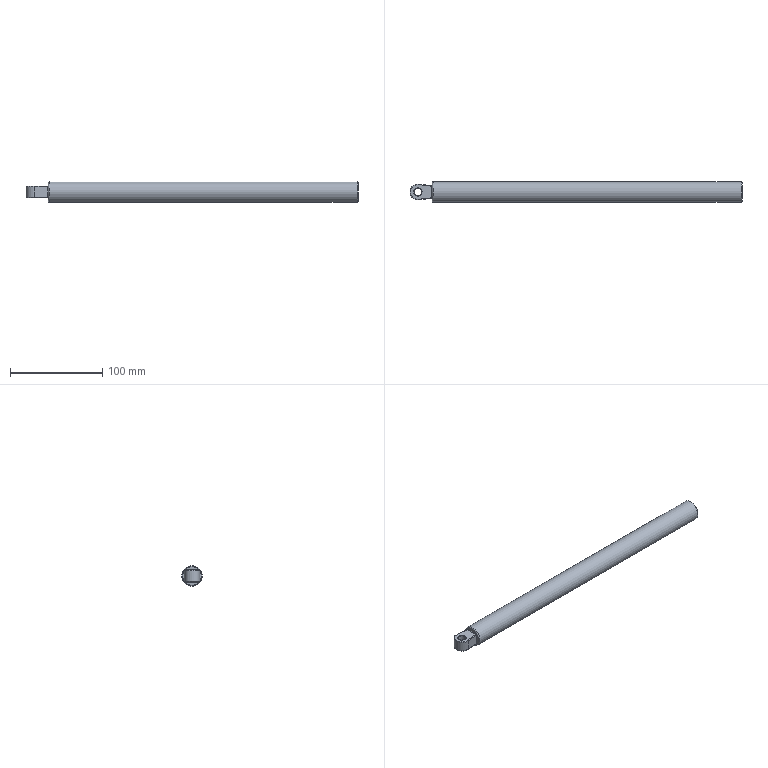Part | STEP file | GAS SHOCK 608X | 1 solid | 30 faces | box 359 x 22 x 22 mm | volume 94119 mm3 | cylinder 12 | plane 7 | torus 7 | spline 4 | commonest cylinder face diameters 1 x8 8.2 x1 12 x1 17 x1 22 x1
STEP:
#1=CARTESIAN_POINT('',(-180.,10.,0.));
#2=VERTEX_POINT('',#1);
#3=CARTESIAN_POINT('',(-180.,0.,0.));
#4=DIRECTION('',(-1.,0.,0.));
#5=DIRECTION('',(0.,1.,0.));
#6=AXIS2_PLACEMENT_3D('',#3,#4,#5);
#7=CIRCLE('',#6,10.);
#8=EDGE_CURVE('',#2,#2,#7,.T.);
#9=ORIENTED_EDGE('',*,*,#8,.T.);
#10=EDGE_LOOP('',(#9));
#11=FACE_OUTER_BOUND('',#10,.T.);
#12=CARTESIAN_POINT('',(-180.,6.305,6.5));
#13=VERTEX_POINT('',#12);
#14=CARTESIAN_POINT('',(-180.,7.312,5.5));
#15=VERTEX_POINT('',#14);
#16=CARTESIAN_POINT('',(-180.,6.305,6.5));
#17=CARTESIAN_POINT('',(-180.,6.895,6.5));
#18=CARTESIAN_POINT('',(-180.,7.312,6.086));
#19=CARTESIAN_POINT('',(-180.,7.312,5.5));
#20=(BOUNDED_CURVE()B_SPLINE_CURVE(3,(#16,#17,#18,#19),.UNSPECIFIED.,.F.,.F.)B_SPLINE_CURVE_WITH_KNOTS((4,4),(1.571,3.142),.UNSPECIFIED.)CURVE()GEOMETRIC_REPRESENTATION_ITEM()RATIONAL_B_SPLINE_CURVE((1.,0.8047,0.8047,1.))REPRESENTATION_ITEM(''));
#21=EDGE_CURVE('',#13,#15,#20,.T.);
#22=ORIENTED_EDGE('',*,*,#21,.F.);
#23=CARTESIAN_POINT('',(-180.,-6.305,6.5));
#24=VERTEX_POINT('',#23);
#25=CARTESIAN_POINT('',(-180.,0.,6.5));
#26=DIRECTION('',(0.,-1.,0.));
#27=VECTOR('',#26,1000.);
#28=LINE('',#25,#27);
#29=EDGE_CURVE('',#13,#24,#28,.T.);
#30=ORIENTED_EDGE('',*,*,#29,.T.);
#31=CARTESIAN_POINT('',(-180.,-7.312,5.5));
#32=VERTEX_POINT('',#31);
#33=CARTESIAN_POINT('',(-180.,-7.312,5.5));
#34=CARTESIAN_POINT('',(-180.,-7.312,6.086));
#35=CARTESIAN_POINT('',(-180.,-6.895,6.5));
#36=CARTESIAN_POINT('',(-180.,-6.305,6.5));
#37=(BOUNDED_CURVE()B_SPLINE_CURVE(3,(#33,#34,#35,#36),.UNSPECIFIED.,.F.,.F.)B_SPLINE_CURVE_WITH_KNOTS((4,4),(0.,1.571),.UNSPECIFIED.)CURVE()GEOMETRIC_REPRESENTATION_ITEM()RATIONAL_B_SPLINE_CURVE((1.,0.8047,0.8047,1.))REPRESENTATION_ITEM(''));
#38=EDGE_CURVE('',#32,#24,#37,.T.);
#39=ORIENTED_EDGE('',*,*,#38,.F.);
#40=CARTESIAN_POINT('',(-180.,-7.312,-5.5));
#41=VERTEX_POINT('',#40);
#42=CARTESIAN_POINT('',(-180.,-7.312,-6.));
#43=DIRECTION('',(0.,0.,-1.));
#44=VECTOR('',#43,1000.);
#45=LINE('',#42,#44);
#46=EDGE_CURVE('',#32,#41,#45,.T.);
#47=ORIENTED_EDGE('',*,*,#46,.T.);
#48=CARTESIAN_POINT('',(-180.,-6.305,-6.5));
#49=VERTEX_POINT('',#48);
#50=CARTESIAN_POINT('',(-180.,-6.305,-6.5));
#51=CARTESIAN_POINT('',(-180.,-6.895,-6.5));
#52=CARTESIAN_POINT('',(-180.,-7.312,-6.086));
#53=CARTESIAN_POINT('',(-180.,-7.312,-5.5));
#54=(BOUNDED_CURVE()B_SPLINE_CURVE(3,(#50,#51,#52,#53),.UNSPECIFIED.,.F.,.F.)B_SPLINE_CURVE_WITH_KNOTS((4,4),(1.571,3.142),.UNSPECIFIED.)CURVE()GEOMETRIC_REPRESENTATION_ITEM()RATIONAL_B_SPLINE_CURVE((1.,0.8047,0.8047,1.))REPRESENTATION_ITEM(''));
#55=EDGE_CURVE('',#49,#41,#54,.T.);
#56=ORIENTED_EDGE('',*,*,#55,.F.);
#57=CARTESIAN_POINT('',(-180.,6.305,-6.5));
#58=VERTEX_POINT('',#57);
#59=CARTESIAN_POINT('',(-180.,6.75,-6.5));
#60=DIRECTION('',(0.,1.,0.));
#61=VECTOR('',#60,1000.);
#62=LINE('',#59,#61);
#63=EDGE_CURVE('',#49,#58,#62,.T.);
#64=ORIENTED_EDGE('',*,*,#63,.T.);
#65=CARTESIAN_POINT('',(-180.,7.312,-5.5));
#66=VERTEX_POINT('',#65);
#67=CARTESIAN_POINT('',(-180.,7.312,-5.5));
#68=CARTESIAN_POINT('',(-180.,7.312,-6.086));
#69=CARTESIAN_POINT('',(-180.,6.895,-6.5));
#70=CARTESIAN_POINT('',(-180.,6.305,-6.5));
#71=(BOUNDED_CURVE()B_SPLINE_CURVE(3,(#67,#68,#69,#70),.UNSPECIFIED.,.F.,.F.)B_SPLINE_CURVE_WITH_KNOTS((4,4),(0.,1.571),.UNSPECIFIED.)CURVE()GEOMETRIC_REPRESENTATION_ITEM()RATIONAL_B_SPLINE_CURVE((1.,0.8047,0.8047,1.))REPRESENTATION_ITEM(''));
#72=EDGE_CURVE('',#66,#58,#71,.T.);
#73=ORIENTED_EDGE('',*,*,#72,.F.);
#74=CARTESIAN_POINT('',(-180.,7.312,6.));
#75=DIRECTION('',(0.,0.,1.));
#76=VECTOR('',#75,1000.);
#77=LINE('',#74,#76);
#78=EDGE_CURVE('',#66,#15,#77,.T.);
#79=ORIENTED_EDGE('',*,*,#78,.T.);
#80=EDGE_LOOP('',(#22,#30,#39,#47,#56,#64,#73,#79));
#81=FACE_BOUND('',#80,.T.);
#82=CARTESIAN_POINT('',(-180.,0.,0.));
#83=DIRECTION('',(1.,0.,0.));
#84=DIRECTION('',(0.,1.,0.));
#85=AXIS2_PLACEMENT_3D('',#82,#83,#84);
#86=PLANE('',#85);
#87=ADVANCED_FACE('',(#11,#81),#86,.F.);
#88=CARTESIAN_POINT('',(155.,-10.,0.));
#89=VERTEX_POINT('',#88);
#90=CARTESIAN_POINT('',(155.,0.,0.));
#91=DIRECTION('',(1.,0.,0.));
#92=DIRECTION('',(0.,-1.,0.));
#93=AXIS2_PLACEMENT_3D('',#90,#91,#92);
#94=CIRCLE('',#93,10.);
#95=EDGE_CURVE('',#89,#89,#94,.T.);
#96=ORIENTED_EDGE('',*,*,#95,.T.);
#97=EDGE_LOOP('',(#96));
#98=FACE_OUTER_BOUND('',#97,.T.);
#99=CARTESIAN_POINT('',(155.,-7.,0.));
#100=VERTEX_POINT('',#99);
#101=CARTESIAN_POINT('',(155.,0.,0.));
#102=DIRECTION('',(-1.,0.,0.));
#103=DIRECTION('',(0.,-1.,0.));
#104=AXIS2_PLACEMENT_3D('',#101,#102,#103);
#105=CIRCLE('',#104,7.);
#106=EDGE_CURVE('',#100,#100,#105,.T.);
#107=ORIENTED_EDGE('',*,*,#106,.T.);
#108=EDGE_LOOP('',(#107));
#109=FACE_BOUND('',#108,.T.);
#110=CARTESIAN_POINT('',(155.,-6.,0.));
#111=DIRECTION('',(-1.,0.,0.));
#112=DIRECTION('',(0.,-1.,0.));
#113=AXIS2_PLACEMENT_3D('',#110,#111,#112);
#114=PLANE('',#113);
#115=ADVANCED_FACE('',(#98,#109),#114,.F.);
#116=CARTESIAN_POINT('',(154.,-6.,0.));
#117=VERTEX_POINT('',#116);
#118=CARTESIAN_POINT('',(154.,0.,0.));
#119=DIRECTION('',(1.,0.,0.));
#120=DIRECTION('',(0.,-1.,0.));
#121=AXIS2_PLACEMENT_3D('',#118,#119,#120);
#122=CIRCLE('',#121,6.);
#123=EDGE_CURVE('',#117,#117,#122,.T.);
#124=ORIENTED_EDGE('',*,*,#123,.T.);
#125=EDGE_LOOP('',(#124));
#126=FACE_OUTER_BOUND('',#125,.T.);
#127=CARTESIAN_POINT('',(-170.,6.,0.));
#128=VERTEX_POINT('',#127);
#129=CARTESIAN_POINT('',(-170.,0.,0.));
#130=DIRECTION('',(1.,0.,0.));
#131=DIRECTION('',(0.,1.,0.));
#132=AXIS2_PLACEMENT_3D('',#129,#130,#131);
#133=CIRCLE('',#132,6.);
#134=EDGE_CURVE('',#128,#128,#133,.T.);
#135=ORIENTED_EDGE('',*,*,#134,.F.);
#136=EDGE_LOOP('',(#135));
#137=FACE_OUTER_BOUND('',#136,.T.);
#138=CARTESIAN_POINT('',(359.975,0.,0.));
#139=DIRECTION('',(1.,0.,0.));
#140=DIRECTION('',(0.,1.,0.));
#141=AXIS2_PLACEMENT_3D('',#138,#139,#140);
#142=CYLINDRICAL_SURFACE('',#141,6.);
#143=ADVANCED_FACE('',(#126,#137),#142,.F.);
#144=ORIENTED_EDGE('',*,*,#134,.T.);
#145=EDGE_LOOP('',(#144));
#146=FACE_OUTER_BOUND('',#145,.T.);
#147=CARTESIAN_POINT('',(-170.,0.,0.));
#148=DIRECTION('',(-1.,0.,0.));
#149=DIRECTION('',(0.,-1.,0.));
#150=AXIS2_PLACEMENT_3D('',#147,#148,#149);
#151=PLANE('',#150);
#152=ADVANCED_FACE('',(#146),#151,.F.);
#153=CARTESIAN_POINT('',(154.,-11.,0.));
#154=VERTEX_POINT('',#153);
#155=CARTESIAN_POINT('',(154.,0.,0.));
#156=DIRECTION('',(-1.,0.,0.));
#157=DIRECTION('',(0.,-1.,0.));
#158=AXIS2_PLACEMENT_3D('',#155,#156,#157);
#159=CIRCLE('',#158,11.);
#160=EDGE_CURVE('',#154,#154,#159,.T.);
#161=ORIENTED_EDGE('',*,*,#160,.T.);
#162=EDGE_LOOP('',(#161));
#163=FACE_OUTER_BOUND('',#162,.T.);
#164=CARTESIAN_POINT('',(-179.,11.,0.));
#165=VERTEX_POINT('',#164);
#166=CARTESIAN_POINT('',(-179.,0.,0.));
#167=DIRECTION('',(1.,0.,0.));
#168=DIRECTION('',(0.,1.,0.));
#169=AXIS2_PLACEMENT_3D('',#166,#167,#168);
#170=CIRCLE('',#169,11.);
#171=EDGE_CURVE('',#165,#165,#170,.T.);
#172=ORIENTED_EDGE('',*,*,#171,.T.);
#173=EDGE_LOOP('',(#172));
#174=FACE_OUTER_BOUND('',#173,.T.);
#175=CARTESIAN_POINT('',(359.975,0.,0.));
#176=DIRECTION('',(1.,0.,0.));
#177=DIRECTION('',(0.,1.,0.));
#178=AXIS2_PLACEMENT_3D('',#175,#176,#177);
#179=CYLINDRICAL_SURFACE('',#178,11.);
#180=ADVANCED_FACE('',(#163,#174),#179,.T.);
#181=ORIENTED_EDGE('',*,*,#160,.F.);
#182=EDGE_LOOP('',(#181));
#183=FACE_OUTER_BOUND('',#182,.T.);
#184=ORIENTED_EDGE('',*,*,#95,.F.);
#185=EDGE_LOOP('',(#184));
#186=FACE_OUTER_BOUND('',#185,.T.);
#187=CARTESIAN_POINT('',(154.,0.,0.));
#188=DIRECTION('',(-1.,0.,0.));
#189=DIRECTION('',(0.,-1.,0.));
#190=AXIS2_PLACEMENT_3D('',#187,#188,#189);
#191=TOROIDAL_SURFACE('',#190,10.,1.);
#192=ADVANCED_FACE('',(#183,#186),#191,.T.);
#193=ORIENTED_EDGE('',*,*,#106,.F.);
#194=EDGE_LOOP('',(#193));
#195=FACE_OUTER_BOUND('',#194,.T.);
#196=ORIENTED_EDGE('',*,*,#123,.F.);
#197=EDGE_LOOP('',(#196));
#198=FACE_OUTER_BOUND('',#197,.T.);
#199=CARTESIAN_POINT('',(154.,0.,0.));
#200=DIRECTION('',(-1.,0.,0.));
#201=DIRECTION('',(0.,-1.,0.));
#202=AXIS2_PLACEMENT_3D('',#199,#200,#201);
#203=TOROIDAL_SURFACE('',#202,7.,1.);
#204=ADVANCED_FACE('',(#195,#198),#203,.T.);
#205=ORIENTED_EDGE('',*,*,#8,.F.);
#206=EDGE_LOOP('',(#205));
#207=FACE_OUTER_BOUND('',#206,.T.);
#208=ORIENTED_EDGE('',*,*,#171,.F.);
#209=EDGE_LOOP('',(#208));
#210=FACE_OUTER_BOUND('',#209,.T.);
#211=CARTESIAN_POINT('',(-179.,0.,0.));
#212=DIRECTION('',(1.,0.,0.));
#213=DIRECTION('',(0.,1.,0.));
#214=AXIS2_PLACEMENT_3D('',#211,#212,#213);
#215=TOROIDAL_SURFACE('',#214,10.,1.);
#216=ADVANCED_FACE('',(#207,#210),#215,.T.);
#217=CARTESIAN_POINT('',(-190.9,0.,6.));
#218=VERTEX_POINT('',#217);
#219=CARTESIAN_POINT('',(-195.5,0.,6.));
#220=DIRECTION('',(0.,0.,-1.));
#221=DIRECTION('',(1.,0.,0.));
#222=AXIS2_PLACEMENT_3D('',#219,#220,#221);
#223=CIRCLE('',#222,4.6);
#224=EDGE_CURVE('',#218,#218,#223,.T.);
#225=ORIENTED_EDGE('',*,*,#224,.T.);
#226=EDGE_LOOP('',(#225));
#227=FACE_BOUND('',#226,.T.);
#228=CARTESIAN_POINT('',(-194.573,7.946,6.));
#229=VERTEX_POINT('',#228);
#230=CARTESIAN_POINT('',(-194.573,-7.946,6.));
#231=VERTEX_POINT('',#230);
#232=CARTESIAN_POINT('',(-195.5,0.,6.));
#233=DIRECTION('',(0.,0.,1.));
#234=DIRECTION('',(1.,0.,0.));
#235=AXIS2_PLACEMENT_3D('',#232,#233,#234);
#236=CIRCLE('',#235,8.);
#237=EDGE_CURVE('',#229,#231,#236,.T.);
#238=ORIENTED_EDGE('',*,*,#237,.T.);
#239=CARTESIAN_POINT('',(-180.5,-6.305,6.));
#240=VERTEX_POINT('',#239);
#241=CARTESIAN_POINT('',(-180.058,-6.253,6.));
#242=DIRECTION('',(0.9933,0.1158,0.));
#243=VECTOR('',#242,1000.);
#244=LINE('',#241,#243);
#245=EDGE_CURVE('',#231,#240,#244,.T.);
#246=ORIENTED_EDGE('',*,*,#245,.T.);
#247=CARTESIAN_POINT('',(-180.5,6.305,6.));
#248=VERTEX_POINT('',#247);
#249=CARTESIAN_POINT('',(-180.5,0.,6.));
#250=DIRECTION('',(0.,1.,0.));
#251=VECTOR('',#250,1000.);
#252=LINE('',#249,#251);
#253=EDGE_CURVE('',#240,#248,#252,.T.);
#254=ORIENTED_EDGE('',*,*,#253,.T.);
#255=CARTESIAN_POINT('',(-194.573,7.946,6.));
#256=DIRECTION('',(-0.9933,0.1158,0.));
#257=VECTOR('',#256,1000.);
#258=LINE('',#255,#257);
#259=EDGE_CURVE('',#248,#229,#258,.T.);
#260=ORIENTED_EDGE('',*,*,#259,.T.);
#261=EDGE_LOOP('',(#238,#246,#254,#260));
#262=FACE_OUTER_BOUND('',#261,.T.);
#263=CARTESIAN_POINT('',(-195.5,0.,6.));
#264=DIRECTION('',(0.,0.,1.));
#265=DIRECTION('',(1.,0.,0.));
#266=AXIS2_PLACEMENT_3D('',#263,#264,#265);
#267=PLANE('',#266);
#268=ADVANCED_FACE('',(#227,#262),#267,.T.);
#269=CARTESIAN_POINT('',(-190.9,0.,-6.));
#270=VERTEX_POINT('',#269);
#271=CARTESIAN_POINT('',(-195.5,0.,-6.));
#272=DIRECTION('',(0.,0.,1.));
#273=DIRECTION('',(1.,0.,0.));
#274=AXIS2_PLACEMENT_3D('',#271,#272,#273);
#275=CIRCLE('',#274,4.6);
#276=EDGE_CURVE('',#270,#270,#275,.T.);
#277=ORIENTED_EDGE('',*,*,#276,.T.);
#278=EDGE_LOOP('',(#277));
#279=FACE_BOUND('',#278,.T.);
#280=CARTESIAN_POINT('',(-194.573,-7.946,-6.));
#281=VERTEX_POINT('',#280);
#282=CARTESIAN_POINT('',(-194.573,7.946,-6.));
#283=VERTEX_POINT('',#282);
#284=CARTESIAN_POINT('',(-195.5,0.,-6.));
#285=DIRECTION('',(0.,0.,-1.));
#286=DIRECTION('',(1.,0.,0.));
#287=AXIS2_PLACEMENT_3D('',#284,#285,#286);
#288=CIRCLE('',#287,8.);
#289=EDGE_CURVE('',#281,#283,#288,.T.);
#290=ORIENTED_EDGE('',*,*,#289,.T.);
#291=CARTESIAN_POINT('',(-180.5,6.305,-6.));
#292=VERTEX_POINT('',#291);
#293=CARTESIAN_POINT('',(-194.573,7.946,-6.));
#294=DIRECTION('',(0.9933,-0.1158,0.));
#295=VECTOR('',#294,1000.);
#296=LINE('',#293,#295);
#297=EDGE_CURVE('',#283,#292,#296,.T.);
#298=ORIENTED_EDGE('',*,*,#297,.T.);
#299=CARTESIAN_POINT('',(-180.5,-6.305,-6.));
#300=VERTEX_POINT('',#299);
#301=CARTESIAN_POINT('',(-180.5,-6.75,-6.));
#302=DIRECTION('',(0.,-1.,0.));
#303=VECTOR('',#302,1000.);
#304=LINE('',#301,#303);
#305=EDGE_CURVE('',#292,#300,#304,.T.);
#306=ORIENTED_EDGE('',*,*,#305,.T.);
#307=CARTESIAN_POINT('',(-194.573,-7.946,-6.));
#308=DIRECTION('',(-0.9933,-0.1158,0.));
#309=VECTOR('',#308,1000.);
#310=LINE('',#307,#309);
#311=EDGE_CURVE('',#300,#281,#310,.T.);
#312=ORIENTED_EDGE('',*,*,#311,.T.);
#313=EDGE_LOOP('',(#290,#298,#306,#312));
#314=FACE_OUTER_BOUND('',#313,.T.);
#315=CARTESIAN_POINT('',(-195.5,0.,-6.));
#316=DIRECTION('',(0.,0.,1.));
#317=DIRECTION('',(1.,0.,0.));
#318=AXIS2_PLACEMENT_3D('',#315,#316,#317);
#319=PLANE('',#318);
#320=ADVANCED_FACE('',(#279,#314),#319,.F.);
#321=CARTESIAN_POINT('',(-194.515,8.443,5.5));
#322=VERTEX_POINT('',#321);
#323=CARTESIAN_POINT('',(-194.515,8.443,-5.5));
#324=VERTEX_POINT('',#323);
#325=CARTESIAN_POINT('',(-194.515,8.443,6.));
#326=DIRECTION('',(0.,0.,-1.));
#327=VECTOR('',#326,1000.);
#328=LINE('',#325,#327);
#329=EDGE_CURVE('',#322,#324,#328,.T.);
#330=ORIENTED_EDGE('',*,*,#329,.F.);
#331=CARTESIAN_POINT('',(-180.558,6.815,5.5));
#332=VERTEX_POINT('',#331);
#333=CARTESIAN_POINT('',(-180.,6.75,5.5));
#334=DIRECTION('',(0.9933,-0.1158,0.));
#335=VECTOR('',#334,1000.);
#336=LINE('',#333,#335);
#337=EDGE_CURVE('',#322,#332,#336,.T.);
#338=ORIENTED_EDGE('',*,*,#337,.T.);
#339=CARTESIAN_POINT('',(-180.558,6.815,-5.5));
#340=VERTEX_POINT('',#339);
#341=CARTESIAN_POINT('',(-180.558,6.815,-6.));
#342=DIRECTION('',(0.,0.,-1.));
#343=VECTOR('',#342,1000.);
#344=LINE('',#341,#343);
#345=EDGE_CURVE('',#332,#340,#344,.T.);
#346=ORIENTED_EDGE('',*,*,#345,.T.);
#347=CARTESIAN_POINT('',(-194.515,8.443,-5.5));
#348=DIRECTION('',(-0.9933,0.1158,0.));
#349=VECTOR('',#348,1000.);
#350=LINE('',#347,#349);
#351=EDGE_CURVE('',#340,#324,#350,.T.);
#352=ORIENTED_EDGE('',*,*,#351,.T.);
#353=EDGE_LOOP('',(#330,#338,#346,#352));
#354=FACE_OUTER_BOUND('',#353,.T.);
#355=CARTESIAN_POINT('',(-194.515,8.443,6.));
#356=DIRECTION('',(-0.1158,-0.9933,0.));
#357=DIRECTION('',(0.9933,-0.1158,0.));
#358=AXIS2_PLACEMENT_3D('',#355,#356,#357);
#359=PLANE('',#358);
#360=ADVANCED_FACE('',(#354),#359,.F.);
#361=CARTESIAN_POINT('',(-194.515,-8.443,5.5));
#362=VERTEX_POINT('',#361);
#363=CARTESIAN_POINT('',(-194.515,-8.443,-5.5));
#364=VERTEX_POINT('',#363);
#365=CARTESIAN_POINT('',(-194.515,-8.443,6.));
#366=DIRECTION('',(0.,0.,-1.));
#367=VECTOR('',#366,1000.);
#368=LINE('',#365,#367);
#369=EDGE_CURVE('',#362,#364,#368,.T.);
#370=ORIENTED_EDGE('',*,*,#369,.F.);
#371=CARTESIAN_POINT('',(-195.5,0.,5.5));
#372=DIRECTION('',(0.,0.,-1.));
#373=DIRECTION('',(1.,0.,0.));
#374=AXIS2_PLACEMENT_3D('',#371,#372,#373);
#375=CIRCLE('',#374,8.5);
#376=EDGE_CURVE('',#362,#322,#375,.T.);
#377=ORIENTED_EDGE('',*,*,#376,.T.);
#378=ORIENTED_EDGE('',*,*,#329,.T.);
#379=CARTESIAN_POINT('',(-195.5,0.,-5.5));
#380=DIRECTION('',(0.,0.,1.));
#381=DIRECTION('',(1.,0.,0.));
#382=AXIS2_PLACEMENT_3D('',#379,#380,#381);
#383=CIRCLE('',#382,8.5);
#384=EDGE_CURVE('',#324,#364,#383,.T.);
#385=ORIENTED_EDGE('',*,*,#384,.T.);
#386=EDGE_LOOP('',(#370,#377,#378,#385));
#387=FACE_OUTER_BOUND('',#386,.T.);
#388=CARTESIAN_POINT('',(-195.5,0.,6.));
#389=DIRECTION('',(0.,0.,-1.));
#390=DIRECTION('',(-1.,0.,0.));
#391=AXIS2_PLACEMENT_3D('',#388,#389,#390);
#392=CYLINDRICAL_SURFACE('',#391,8.5);
#393=ADVANCED_FACE('',(#387),#392,.T.);
#394=CARTESIAN_POINT('',(-180.558,-6.815,-5.5));
#395=VERTEX_POINT('',#394);
#396=CARTESIAN_POINT('',(-180.558,-6.815,5.5));
#397=VERTEX_POINT('',#396);
#398=CARTESIAN_POINT('',(-180.558,-6.815,6.));
#399=DIRECTION('',(0.,0.,1.));
#400=VECTOR('',#399,1000.);
#401=LINE('',#398,#400);
#402=EDGE_CURVE('',#395,#397,#401,.T.);
#403=ORIENTED_EDGE('',*,*,#402,.T.);
#404=CARTESIAN_POINT('',(-194.515,-8.443,5.5));
#405=DIRECTION('',(-0.9933,-0.1158,0.));
#406=VECTOR('',#405,1000.);
#407=LINE('',#404,#406);
#408=EDGE_CURVE('',#397,#362,#407,.T.);
#409=ORIENTED_EDGE('',*,*,#408,.T.);
#410=ORIENTED_EDGE('',*,*,#369,.T.);
#411=CARTESIAN_POINT('',(-194.515,-8.443,-5.5));
#412=DIRECTION('',(0.9933,0.1158,0.));
#413=VECTOR('',#412,1000.);
#414=LINE('',#411,#413);
#415=EDGE_CURVE('',#364,#395,#414,.T.);
#416=ORIENTED_EDGE('',*,*,#415,.T.);
#417=EDGE_LOOP('',(#403,#409,#410,#416));
#418=FACE_OUTER_BOUND('',#417,.T.);
#419=CARTESIAN_POINT('',(-194.515,-8.443,6.));
#420=DIRECTION('',(-0.1158,0.9933,0.));
#421=DIRECTION('',(-0.9933,-0.1158,0.));
#422=AXIS2_PLACEMENT_3D('',#419,#420,#421);
#423=PLANE('',#422);
#424=ADVANCED_FACE('',(#418),#423,.F.);
#425=CARTESIAN_POINT('',(-191.4,0.,5.5));
#426=VERTEX_POINT('',#425);
#427=CARTESIAN_POINT('',(-195.5,0.,5.5));
#428=DIRECTION('',(0.,0.,1.));
#429=DIRECTION('',(1.,0.,0.));
#430=AXIS2_PLACEMENT_3D('',#427,#428,#429);
#431=CIRCLE('',#430,4.1);
#432=EDGE_CURVE('',#426,#426,#431,.T.);
#433=ORIENTED_EDGE('',*,*,#432,.T.);
#434=EDGE_LOOP('',(#433));
#435=FACE_OUTER_BOUND('',#434,.T.);
#436=CARTESIAN_POINT('',(-191.4,0.,-5.5));
#437=VERTEX_POINT('',#436);
#438=CARTESIAN_POINT('',(-195.5,0.,-5.5));
#439=DIRECTION('',(0.,0.,-1.));
#440=DIRECTION('',(1.,0.,0.));
#441=AXIS2_PLACEMENT_3D('',#438,#439,#440);
#442=CIRCLE('',#441,4.1);
#443=EDGE_CURVE('',#437,#437,#442,.T.);
#444=ORIENTED_EDGE('',*,*,#443,.T.);
#445=EDGE_LOOP('',(#444));
#446=FACE_OUTER_BOUND('',#445,.T.);
#447=CARTESIAN_POINT('',(-195.5,0.,6.));
#448=DIRECTION('',(0.,0.,-1.));
#449=DIRECTION('',(-1.,0.,0.));
#450=AXIS2_PLACEMENT_3D('',#447,#448,#449);
#451=CYLINDRICAL_SURFACE('',#450,4.1);
#452=ADVANCED_FACE('',(#435,#446),#451,.F.);
#453=CARTESIAN_POINT('',(-194.573,-7.946,5.5));
#454=DIRECTION('',(-0.9933,-0.1158,0.));
#455=DIRECTION('',(0.1158,-0.9933,0.));
#456=AXIS2_PLACEMENT_3D('',#453,#454,#455);
#457=CIRCLE('',#456,0.5);
#458=EDGE_CURVE('',#362,#231,#457,.T.);
#459=ORIENTED_EDGE('',*,*,#458,.F.);
#460=ORIENTED_EDGE('',*,*,#408,.F.);
#461=CARTESIAN_POINT('',(-180.5,-6.305,6.));
#462=CARTESIAN_POINT('',(-180.534,-6.604,6.));
#463=CARTESIAN_POINT('',(-180.558,-6.815,5.793));
#464=CARTESIAN_POINT('',(-180.558,-6.815,5.5));
#465=(BOUNDED_CURVE()B_SPLINE_CURVE(3,(#461,#462,#463,#464),.UNSPECIFIED.,.F.,.F.)B_SPLINE_CURVE_WITH_KNOTS((4,4),(4.712,6.283),.UNSPECIFIED.)CURVE()GEOMETRIC_REPRESENTATION_ITEM()RATIONAL_B_SPLINE_CURVE((1.,0.8047,0.8047,1.))REPRESENTATION_ITEM(''));
#466=EDGE_CURVE('',#240,#397,#465,.T.);
#467=ORIENTED_EDGE('',*,*,#466,.F.);
#468=ORIENTED_EDGE('',*,*,#245,.F.);
#469=EDGE_LOOP('',(#459,#460,#467,#468));
#470=FACE_OUTER_BOUND('',#469,.T.);
#471=CARTESIAN_POINT('',(-194.573,-7.946,5.5));
#472=DIRECTION('',(-0.9933,-0.1158,0.));
#473=DIRECTION('',(0.1158,-0.9933,0.));
#474=AXIS2_PLACEMENT_3D('',#471,#472,#473);
#475=CYLINDRICAL_SURFACE('',#474,0.5);
#476=ADVANCED_FACE('',(#470),#475,.T.);
#477=CARTESIAN_POINT('',(-180.558,-6.815,-5.5));
#478=CARTESIAN_POINT('',(-180.558,-6.815,-5.793));
#479=CARTESIAN_POINT('',(-180.534,-6.604,-6.));
#480=CARTESIAN_POINT('',(-180.5,-6.305,-6.));
#481=(BOUNDED_CURVE()B_SPLINE_CURVE(3,(#477,#478,#479,#480),.UNSPECIFIED.,.F.,.F.)B_SPLINE_CURVE_WITH_KNOTS((4,4),(3.142,4.712),.UNSPECIFIED.)CURVE()GEOMETRIC_REPRESENTATION_ITEM()RATIONAL_B_SPLINE_CURVE((1.,0.8047,0.8047,1.))REPRESENTATION_ITEM(''));
#482=EDGE_CURVE('',#395,#300,#481,.T.);
#483=ORIENTED_EDGE('',*,*,#482,.F.);
#484=ORIENTED_EDGE('',*,*,#415,.F.);
#485=CARTESIAN_POINT('',(-194.573,-7.946,-5.5));
#486=DIRECTION('',(-0.9933,-0.1158,0.));
#487=DIRECTION('',(0.1158,-0.9933,0.));
#488=AXIS2_PLACEMENT_3D('',#485,#486,#487);
#489=CIRCLE('',#488,0.5);
#490=EDGE_CURVE('',#281,#364,#489,.T.);
#491=ORIENTED_EDGE('',*,*,#490,.F.);
#492=ORIENTED_EDGE('',*,*,#311,.F.);
#493=EDGE_LOOP('',(#483,#484,#491,#492));
#494=FACE_OUTER_BOUND('',#493,.T.);
#495=CARTESIAN_POINT('',(-194.573,-7.946,-5.5));
#496=DIRECTION('',(0.9933,0.1158,0.));
#497=DIRECTION('',(-0.1158,0.9933,0.));
#498=AXIS2_PLACEMENT_3D('',#495,#496,#497);
#499=CYLINDRICAL_SURFACE('',#498,0.5);
#500=ADVANCED_FACE('',(#494),#499,.T.);
#501=CARTESIAN_POINT('',(-180.5,-7.312,-5.5));
#502=DIRECTION('',(0.,0.,1.));
#503=DIRECTION('',(1.,0.,0.));
#504=AXIS2_PLACEMENT_3D('',#501,#502,#503);
#505=CIRCLE('',#504,0.5);
#506=EDGE_CURVE('',#41,#395,#505,.T.);
#507=ORIENTED_EDGE('',*,*,#506,.F.);
#508=ORIENTED_EDGE('',*,*,#46,.F.);
#509=CARTESIAN_POINT('',(-180.5,-7.312,5.5));
#510=DIRECTION('',(0.,0.,-1.));
#511=DIRECTION('',(-1.,0.,0.));
#512=AXIS2_PLACEMENT_3D('',#509,#510,#511);
#513=CIRCLE('',#512,0.5);
#514=EDGE_CURVE('',#397,#32,#513,.T.);
#515=ORIENTED_EDGE('',*,*,#514,.F.);
#516=ORIENTED_EDGE('',*,*,#402,.F.);
#517=EDGE_LOOP('',(#507,#508,#515,#516));
#518=FACE_OUTER_BOUND('',#517,.T.);
#519=CARTESIAN_POINT('',(-180.5,-7.312,0.));
#520=DIRECTION('',(0.,0.,1.));
#521=DIRECTION('',(1.,0.,0.));
#522=AXIS2_PLACEMENT_3D('',#519,#520,#521);
#523=CYLINDRICAL_SURFACE('',#522,0.5);
#524=ADVANCED_FACE('',(#518),#523,.F.);
#525=ORIENTED_EDGE('',*,*,#514,.T.);
#526=ORIENTED_EDGE('',*,*,#38,.T.);
#527=CARTESIAN_POINT('',(-180.5,-6.305,6.5));
#528=DIRECTION('',(0.,-1.,0.));
#529=DIRECTION('',(0.,0.,1.));
#530=AXIS2_PLACEMENT_3D('',#527,#528,#529);
#531=CIRCLE('',#530,0.5);
#532=EDGE_CURVE('',#240,#24,#531,.T.);
#533=ORIENTED_EDGE('',*,*,#532,.F.);
#534=ORIENTED_EDGE('',*,*,#466,.T.);
#535=EDGE_LOOP('',(#525,#526,#533,#534));
#536=FACE_OUTER_BOUND('',#535,.T.);
#537=CARTESIAN_POINT('',(-180.,-6.305,6.5));
#538=CARTESIAN_POINT('',(-180.,-6.305,6.));
#539=CARTESIAN_POINT('',(-180.5,-6.305,6.));
#540=CARTESIAN_POINT('',(-180.,-6.569,6.5));
#541=CARTESIAN_POINT('',(-180.,-6.442,5.984));
#542=CARTESIAN_POINT('',(-180.515,-6.439,6.));
#543=CARTESIAN_POINT('',(-180.,-6.83,6.392));
#544=CARTESIAN_POINT('',(-180.,-6.558,5.914));
#545=CARTESIAN_POINT('',(-180.53,-6.571,5.946));
#546=CARTESIAN_POINT('',(-180.,-7.203,6.022));
#547=CARTESIAN_POINT('',(-180.,-6.713,5.728));
#548=CARTESIAN_POINT('',(-180.552,-6.76,5.761));
#549=CARTESIAN_POINT('',(-180.,-7.312,5.763));
#550=CARTESIAN_POINT('',(-180.,-6.75,5.613));
#551=CARTESIAN_POINT('',(-180.558,-6.815,5.631));
#552=CARTESIAN_POINT('',(-180.,-7.312,5.5));
#553=CARTESIAN_POINT('',(-180.,-6.75,5.5));
#554=CARTESIAN_POINT('',(-180.558,-6.815,5.5));
#555=(BOUNDED_SURFACE()B_SPLINE_SURFACE(3,2,((#537,#538,#539),(#540,#541,#542),(#543,#544,#545),(#546,#547,#548),(#549,#550,#551),(#552,#553,#554)),.UNSPECIFIED.,.F.,.F.,.T.)B_SPLINE_SURFACE_WITH_KNOTS((4,2,4),(3,3),(4.712,5.498,6.283),(0.,1.),.UNSPECIFIED.)GEOMETRIC_REPRESENTATION_ITEM()RATIONAL_B_SPLINE_SURFACE(((1.,0.7071,1.),(1.,0.6964,1.),(1.,0.6854,1.),(1.,0.6696,1.),(1.,0.6648,1.),(1.,0.6649,1.)))REPRESENTATION_ITEM('')SURFACE());
#556=ADVANCED_FACE('',(#536),#555,.F.);
#557=ORIENTED_EDGE('',*,*,#458,.T.);
#558=ORIENTED_EDGE('',*,*,#237,.F.);
#559=CARTESIAN_POINT('',(-194.573,7.946,5.5));
#560=DIRECTION('',(0.9933,-0.1158,0.));
#561=DIRECTION('',(0.1158,0.9933,0.));
#562=AXIS2_PLACEMENT_3D('',#559,#560,#561);
#563=CIRCLE('',#562,0.5);
#564=EDGE_CURVE('',#322,#229,#563,.T.);
#565=ORIENTED_EDGE('',*,*,#564,.F.);
#566=ORIENTED_EDGE('',*,*,#376,.F.);
#567=EDGE_LOOP('',(#557,#558,#565,#566));
#568=FACE_OUTER_BOUND('',#567,.T.);
#569=CARTESIAN_POINT('',(-195.5,0.,5.5));
#570=DIRECTION('',(0.,0.,1.));
#571=DIRECTION('',(1.,0.,0.));
#572=AXIS2_PLACEMENT_3D('',#569,#570,#571);
#573=TOROIDAL_SURFACE('',#572,8.,0.5);
#574=ADVANCED_FACE('',(#568),#573,.T.);
#575=ORIENTED_EDGE('',*,*,#490,.T.);
#576=ORIENTED_EDGE('',*,*,#384,.F.);
#577=CARTESIAN_POINT('',(-194.573,7.946,-5.5));
#578=DIRECTION('',(0.9933,-0.1158,0.));
#579=DIRECTION('',(0.1158,0.9933,0.));
#580=AXIS2_PLACEMENT_3D('',#577,#578,#579);
#581=CIRCLE('',#580,0.5);
#582=EDGE_CURVE('',#283,#324,#581,.T.);
#583=ORIENTED_EDGE('',*,*,#582,.F.);
#584=ORIENTED_EDGE('',*,*,#289,.F.);
#585=EDGE_LOOP('',(#575,#576,#583,#584));
#586=FACE_OUTER_BOUND('',#585,.T.);
#587=CARTESIAN_POINT('',(-195.5,0.,-5.5));
#588=DIRECTION('',(0.,0.,1.));
#589=DIRECTION('',(1.,0.,0.));
#590=AXIS2_PLACEMENT_3D('',#587,#588,#589);
#591=TOROIDAL_SURFACE('',#590,8.,0.5);
#592=ADVANCED_FACE('',(#586),#591,.T.);
#593=ORIENTED_EDGE('',*,*,#506,.T.);
#594=ORIENTED_EDGE('',*,*,#482,.T.);
#595=CARTESIAN_POINT('',(-180.5,-6.305,-6.5));
#596=DIRECTION('',(0.,-1.,0.));
#597=DIRECTION('',(0.,0.,1.));
#598=AXIS2_PLACEMENT_3D('',#595,#596,#597);
#599=CIRCLE('',#598,0.5);
#600=EDGE_CURVE('',#49,#300,#599,.T.);
#601=ORIENTED_EDGE('',*,*,#600,.F.);
#602=ORIENTED_EDGE('',*,*,#55,.T.);
#603=EDGE_LOOP('',(#593,#594,#601,#602));
#604=FACE_OUTER_BOUND('',#603,.T.);
#605=CARTESIAN_POINT('',(-180.,-7.312,-5.5));
#606=CARTESIAN_POINT('',(-180.,-6.75,-5.5));
#607=CARTESIAN_POINT('',(-180.558,-6.815,-5.5));
#608=CARTESIAN_POINT('',(-180.,-7.312,-5.763));
#609=CARTESIAN_POINT('',(-180.,-6.75,-5.613));
#610=CARTESIAN_POINT('',(-180.558,-6.815,-5.631));
#611=CARTESIAN_POINT('',(-180.,-7.203,-6.022));
#612=CARTESIAN_POINT('',(-180.,-6.713,-5.728));
#613=CARTESIAN_POINT('',(-180.552,-6.76,-5.761));
#614=CARTESIAN_POINT('',(-180.,-6.83,-6.392));
#615=CARTESIAN_POINT('',(-180.,-6.558,-5.914));
#616=CARTESIAN_POINT('',(-180.53,-6.571,-5.946));
#617=CARTESIAN_POINT('',(-180.,-6.569,-6.5));
#618=CARTESIAN_POINT('',(-180.,-6.442,-5.984));
#619=CARTESIAN_POINT('',(-180.515,-6.439,-6.));
#620=CARTESIAN_POINT('',(-180.,-6.305,-6.5));
#621=CARTESIAN_POINT('',(-180.,-6.305,-6.));
#622=CARTESIAN_POINT('',(-180.5,-6.305,-6.));
#623=(BOUNDED_SURFACE()B_SPLINE_SURFACE(3,2,((#605,#606,#607),(#608,#609,#610),(#611,#612,#613),(#614,#615,#616),(#617,#618,#619),(#620,#621,#622)),.UNSPECIFIED.,.F.,.F.,.T.)B_SPLINE_SURFACE_WITH_KNOTS((4,2,4),(3,3),(3.142,3.927,4.712),(0.,1.),.UNSPECIFIED.)GEOMETRIC_REPRESENTATION_ITEM()RATIONAL_B_SPLINE_SURFACE(((1.,0.6649,1.),(1.,0.6648,1.),(1.,0.6696,1.),(1.,0.6854,1.),(1.,0.6964,1.),(1.,0.7071,1.)))REPRESENTATION_ITEM('')SURFACE());
#624=ADVANCED_FACE('',(#604),#623,.F.);
#625=ORIENTED_EDGE('',*,*,#532,.T.);
#626=ORIENTED_EDGE('',*,*,#29,.F.);
#627=CARTESIAN_POINT('',(-180.5,6.305,6.5));
#628=DIRECTION('',(0.,-1.,0.));
#629=DIRECTION('',(0.,0.,-1.));
#630=AXIS2_PLACEMENT_3D('',#627,#628,#629);
#631=CIRCLE('',#630,0.5);
#632=EDGE_CURVE('',#248,#13,#631,.T.);
#633=ORIENTED_EDGE('',*,*,#632,.F.);
#634=ORIENTED_EDGE('',*,*,#253,.F.);
#635=EDGE_LOOP('',(#625,#626,#633,#634));
#636=FACE_OUTER_BOUND('',#635,.T.);
#637=CARTESIAN_POINT('',(-180.5,0.,6.5));
#638=DIRECTION('',(0.,1.,0.));
#639=DIRECTION('',(-1.,0.,0.));
#640=AXIS2_PLACEMENT_3D('',#637,#638,#639);
#641=CYLINDRICAL_SURFACE('',#640,0.5);
#642=ADVANCED_FACE('',(#636),#641,.F.);
#643=ORIENTED_EDGE('',*,*,#564,.T.);
#644=ORIENTED_EDGE('',*,*,#259,.F.);
#645=CARTESIAN_POINT('',(-180.558,6.815,5.5));
#646=CARTESIAN_POINT('',(-180.558,6.815,5.793));
#647=CARTESIAN_POINT('',(-180.534,6.604,6.));
#648=CARTESIAN_POINT('',(-180.5,6.305,6.));
#649=(BOUNDED_CURVE()B_SPLINE_CURVE(3,(#645,#646,#647,#648),.UNSPECIFIED.,.F.,.F.)B_SPLINE_CURVE_WITH_KNOTS((4,4),(3.142,4.712),.UNSPECIFIED.)CURVE()GEOMETRIC_REPRESENTATION_ITEM()RATIONAL_B_SPLINE_CURVE((1.,0.8047,0.8047,1.))REPRESENTATION_ITEM(''));
#650=EDGE_CURVE('',#332,#248,#649,.T.);
#651=ORIENTED_EDGE('',*,*,#650,.F.);
#652=ORIENTED_EDGE('',*,*,#337,.F.);
#653=EDGE_LOOP('',(#643,#644,#651,#652));
#654=FACE_OUTER_BOUND('',#653,.T.);
#655=CARTESIAN_POINT('',(-194.573,7.946,5.5));
#656=DIRECTION('',(0.9933,-0.1158,0.));
#657=DIRECTION('',(0.1158,0.9933,0.));
#658=AXIS2_PLACEMENT_3D('',#655,#656,#657);
#659=CYLINDRICAL_SURFACE('',#658,0.5);
#660=ADVANCED_FACE('',(#654),#659,.T.);
#661=ORIENTED_EDGE('',*,*,#582,.T.);
#662=ORIENTED_EDGE('',*,*,#351,.F.);
#663=CARTESIAN_POINT('',(-180.5,6.305,-6.));
#664=CARTESIAN_POINT('',(-180.534,6.604,-6.));
#665=CARTESIAN_POINT('',(-180.558,6.815,-5.793));
#666=CARTESIAN_POINT('',(-180.558,6.815,-5.5));
#667=(BOUNDED_CURVE()B_SPLINE_CURVE(3,(#663,#664,#665,#666),.UNSPECIFIED.,.F.,.F.)B_SPLINE_CURVE_WITH_KNOTS((4,4),(4.712,6.283),.UNSPECIFIED.)CURVE()GEOMETRIC_REPRESENTATION_ITEM()RATIONAL_B_SPLINE_CURVE((1.,0.8047,0.8047,1.))REPRESENTATION_ITEM(''));
#668=EDGE_CURVE('',#292,#340,#667,.T.);
#669=ORIENTED_EDGE('',*,*,#668,.F.);
#670=ORIENTED_EDGE('',*,*,#297,.F.);
#671=EDGE_LOOP('',(#661,#662,#669,#670));
#672=FACE_OUTER_BOUND('',#671,.T.);
#673=CARTESIAN_POINT('',(-194.573,7.946,-5.5));
#674=DIRECTION('',(-0.9933,0.1158,0.));
#675=DIRECTION('',(-0.1158,-0.9933,0.));
#676=AXIS2_PLACEMENT_3D('',#673,#674,#675);
#677=CYLINDRICAL_SURFACE('',#676,0.5);
#678=ADVANCED_FACE('',(#672),#677,.T.);
#679=ORIENTED_EDGE('',*,*,#600,.T.);
#680=ORIENTED_EDGE('',*,*,#305,.F.);
#681=CARTESIAN_POINT('',(-180.5,6.305,-6.5));
#682=DIRECTION('',(0.,-1.,0.));
#683=DIRECTION('',(0.,0.,-1.));
#684=AXIS2_PLACEMENT_3D('',#681,#682,#683);
#685=CIRCLE('',#684,0.5);
#686=EDGE_CURVE('',#58,#292,#685,.T.);
#687=ORIENTED_EDGE('',*,*,#686,.F.);
#688=ORIENTED_EDGE('',*,*,#63,.F.);
#689=EDGE_LOOP('',(#679,#680,#687,#688));
#690=FACE_OUTER_BOUND('',#689,.T.);
#691=CARTESIAN_POINT('',(-180.5,0.,-6.5));
#692=DIRECTION('',(0.,-1.,0.));
#693=DIRECTION('',(1.,0.,0.));
#694=AXIS2_PLACEMENT_3D('',#691,#692,#693);
#695=CYLINDRICAL_SURFACE('',#694,0.5);
#696=ADVANCED_FACE('',(#690),#695,.F.);
#697=ORIENTED_EDGE('',*,*,#632,.T.);
#698=ORIENTED_EDGE('',*,*,#21,.T.);
#699=CARTESIAN_POINT('',(-180.5,7.312,5.5));
#700=DIRECTION('',(0.,0.,1.));
#701=DIRECTION('',(-1.,0.,0.));
#702=AXIS2_PLACEMENT_3D('',#699,#700,#701);
#703=CIRCLE('',#702,0.5);
#704=EDGE_CURVE('',#332,#15,#703,.T.);
#705=ORIENTED_EDGE('',*,*,#704,.F.);
#706=ORIENTED_EDGE('',*,*,#650,.T.);
#707=EDGE_LOOP('',(#697,#698,#705,#706));
#708=FACE_OUTER_BOUND('',#707,.T.);
#709=CARTESIAN_POINT('',(-180.,7.312,5.5));
#710=CARTESIAN_POINT('',(-180.,6.75,5.5));
#711=CARTESIAN_POINT('',(-180.558,6.815,5.5));
#712=CARTESIAN_POINT('',(-180.,7.312,5.763));
#713=CARTESIAN_POINT('',(-180.,6.75,5.613));
#714=CARTESIAN_POINT('',(-180.558,6.815,5.631));
#715=CARTESIAN_POINT('',(-180.,7.203,6.022));
#716=CARTESIAN_POINT('',(-180.,6.713,5.728));
#717=CARTESIAN_POINT('',(-180.552,6.76,5.761));
#718=CARTESIAN_POINT('',(-180.,6.83,6.392));
#719=CARTESIAN_POINT('',(-180.,6.558,5.914));
#720=CARTESIAN_POINT('',(-180.53,6.571,5.946));
#721=CARTESIAN_POINT('',(-180.,6.569,6.5));
#722=CARTESIAN_POINT('',(-180.,6.442,5.984));
#723=CARTESIAN_POINT('',(-180.515,6.439,6.));
#724=CARTESIAN_POINT('',(-180.,6.305,6.5));
#725=CARTESIAN_POINT('',(-180.,6.305,6.));
#726=CARTESIAN_POINT('',(-180.5,6.305,6.));
#727=(BOUNDED_SURFACE()B_SPLINE_SURFACE(3,2,((#709,#710,#711),(#712,#713,#714),(#715,#716,#717),(#718,#719,#720),(#721,#722,#723),(#724,#725,#726)),.UNSPECIFIED.,.F.,.F.,.T.)B_SPLINE_SURFACE_WITH_KNOTS((4,2,4),(3,3),(3.142,3.927,4.712),(0.,1.),.UNSPECIFIED.)GEOMETRIC_REPRESENTATION_ITEM()RATIONAL_B_SPLINE_SURFACE(((1.,0.6649,1.),(1.,0.6648,1.),(1.,0.6696,1.),(1.,0.6854,1.),(1.,0.6964,1.),(1.,0.7071,1.)))REPRESENTATION_ITEM('')SURFACE());
#728=ADVANCED_FACE('',(#708),#727,.F.);
#729=ORIENTED_EDGE('',*,*,#686,.T.);
#730=ORIENTED_EDGE('',*,*,#668,.T.);
#731=CARTESIAN_POINT('',(-180.5,7.312,-5.5));
#732=DIRECTION('',(0.,0.,-1.));
#733=DIRECTION('',(1.,0.,0.));
#734=AXIS2_PLACEMENT_3D('',#731,#732,#733);
#735=CIRCLE('',#734,0.5);
#736=EDGE_CURVE('',#66,#340,#735,.T.);
#737=ORIENTED_EDGE('',*,*,#736,.F.);
#738=ORIENTED_EDGE('',*,*,#72,.T.);
#739=EDGE_LOOP('',(#729,#730,#737,#738));
#740=FACE_OUTER_BOUND('',#739,.T.);
#741=CARTESIAN_POINT('',(-180.,6.305,-6.5));
#742=CARTESIAN_POINT('',(-180.,6.305,-6.));
#743=CARTESIAN_POINT('',(-180.5,6.305,-6.));
#744=CARTESIAN_POINT('',(-180.,6.569,-6.5));
#745=CARTESIAN_POINT('',(-180.,6.442,-5.984));
#746=CARTESIAN_POINT('',(-180.515,6.439,-6.));
#747=CARTESIAN_POINT('',(-180.,6.83,-6.392));
#748=CARTESIAN_POINT('',(-180.,6.558,-5.914));
#749=CARTESIAN_POINT('',(-180.53,6.571,-5.946));
#750=CARTESIAN_POINT('',(-180.,7.203,-6.022));
#751=CARTESIAN_POINT('',(-180.,6.713,-5.728));
#752=CARTESIAN_POINT('',(-180.552,6.76,-5.761));
#753=CARTESIAN_POINT('',(-180.,7.312,-5.763));
#754=CARTESIAN_POINT('',(-180.,6.75,-5.613));
#755=CARTESIAN_POINT('',(-180.558,6.815,-5.631));
#756=CARTESIAN_POINT('',(-180.,7.312,-5.5));
#757=CARTESIAN_POINT('',(-180.,6.75,-5.5));
#758=CARTESIAN_POINT('',(-180.558,6.815,-5.5));
#759=(BOUNDED_SURFACE()B_SPLINE_SURFACE(3,2,((#741,#742,#743),(#744,#745,#746),(#747,#748,#749),(#750,#751,#752),(#753,#754,#755),(#756,#757,#758)),.UNSPECIFIED.,.F.,.F.,.T.)B_SPLINE_SURFACE_WITH_KNOTS((4,2,4),(3,3),(4.712,5.498,6.283),(0.,1.),.UNSPECIFIED.)GEOMETRIC_REPRESENTATION_ITEM()RATIONAL_B_SPLINE_SURFACE(((1.,0.7071,1.),(1.,0.6964,1.),(1.,0.6854,1.),(1.,0.6696,1.),(1.,0.6648,1.),(1.,0.6649,1.)))REPRESENTATION_ITEM('')SURFACE());
#760=ADVANCED_FACE('',(#740),#759,.F.);
#761=ORIENTED_EDGE('',*,*,#704,.T.);
#762=ORIENTED_EDGE('',*,*,#78,.F.);
#763=ORIENTED_EDGE('',*,*,#736,.T.);
#764=ORIENTED_EDGE('',*,*,#345,.F.);
#765=EDGE_LOOP('',(#761,#762,#763,#764));
#766=FACE_OUTER_BOUND('',#765,.T.);
#767=CARTESIAN_POINT('',(-180.5,7.312,6.));
#768=DIRECTION('',(0.,0.,1.));
#769=DIRECTION('',(1.,0.,0.));
#770=AXIS2_PLACEMENT_3D('',#767,#768,#769);
#771=CYLINDRICAL_SURFACE('',#770,0.5);
#772=ADVANCED_FACE('',(#766),#771,.F.);
#773=ORIENTED_EDGE('',*,*,#224,.F.);
#774=EDGE_LOOP('',(#773));
#775=FACE_OUTER_BOUND('',#774,.T.);
#776=ORIENTED_EDGE('',*,*,#432,.F.);
#777=EDGE_LOOP('',(#776));
#778=FACE_OUTER_BOUND('',#777,.T.);
#779=CARTESIAN_POINT('',(-195.5,0.,5.5));
#780=DIRECTION('',(0.,0.,1.));
#781=DIRECTION('',(1.,0.,0.));
#782=AXIS2_PLACEMENT_3D('',#779,#780,#781);
#783=TOROIDAL_SURFACE('',#782,4.6,0.5);
#784=ADVANCED_FACE('',(#775,#778),#783,.T.);
#785=ORIENTED_EDGE('',*,*,#443,.F.);
#786=EDGE_LOOP('',(#785));
#787=FACE_OUTER_BOUND('',#786,.T.);
#788=ORIENTED_EDGE('',*,*,#276,.F.);
#789=EDGE_LOOP('',(#788));
#790=FACE_OUTER_BOUND('',#789,.T.);
#791=CARTESIAN_POINT('',(-195.5,0.,-5.5));
#792=DIRECTION('',(0.,0.,1.));
#793=DIRECTION('',(1.,0.,0.));
#794=AXIS2_PLACEMENT_3D('',#791,#792,#793);
#795=TOROIDAL_SURFACE('',#794,4.6,0.5);
#796=ADVANCED_FACE('',(#787,#790),#795,.T.);
#797=CLOSED_SHELL('',(#87,#115,#143,#152,#180,#192,#204,#216,#268,#320,#360,#393,#424,#452,#476,#500,#524,#556,#574,#592,#624,#642,#660,#678,#696,#728,#760,#772,#784,#796));
#798=MANIFOLD_SOLID_BREP('',#797);
#799=CARTESIAN_POINT('',(0.,0.,0.));
#800=DIRECTION('',(0.,0.,1.));
#801=DIRECTION('',(1.,0.,0.));
#802=AXIS2_PLACEMENT_3D('',#799,#800,#801);
#803=(LENGTH_UNIT()NAMED_UNIT(*)SI_UNIT(.MILLI.,.METRE.));
#804=UNCERTAINTY_MEASURE_WITH_UNIT(LENGTH_MEASURE(0.00001),#803,'','');
#805=(NAMED_UNIT(*)PLANE_ANGLE_UNIT()SI_UNIT($,.RADIAN.));
#806=(NAMED_UNIT(*)SI_UNIT($,.STERADIAN.)SOLID_ANGLE_UNIT());
#807=(GEOMETRIC_REPRESENTATION_CONTEXT(3)GLOBAL_UNCERTAINTY_ASSIGNED_CONTEXT((#804))GLOBAL_UNIT_ASSIGNED_CONTEXT((#803,#805,#806))REPRESENTATION_CONTEXT('',''));
#808=ADVANCED_BREP_SHAPE_REPRESENTATION('',(#798,#802),#807);